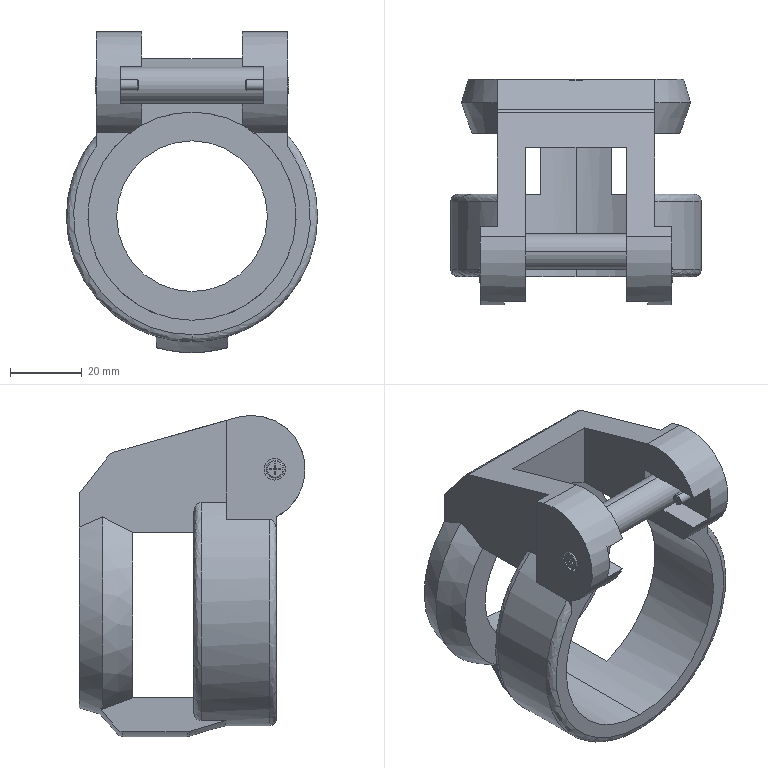Part | STEP file | _CGR01-60-U-002_1 | 1 solid | 126 faces | box 70 x 63 x 89.5 mm | volume 81661 mm3 | plane 61 | cone 32 | cylinder 25 | spline 8 | commonest cylinder face diameters 3 x6 5 x4 6 x4 10 x2 30 x2 42 x2